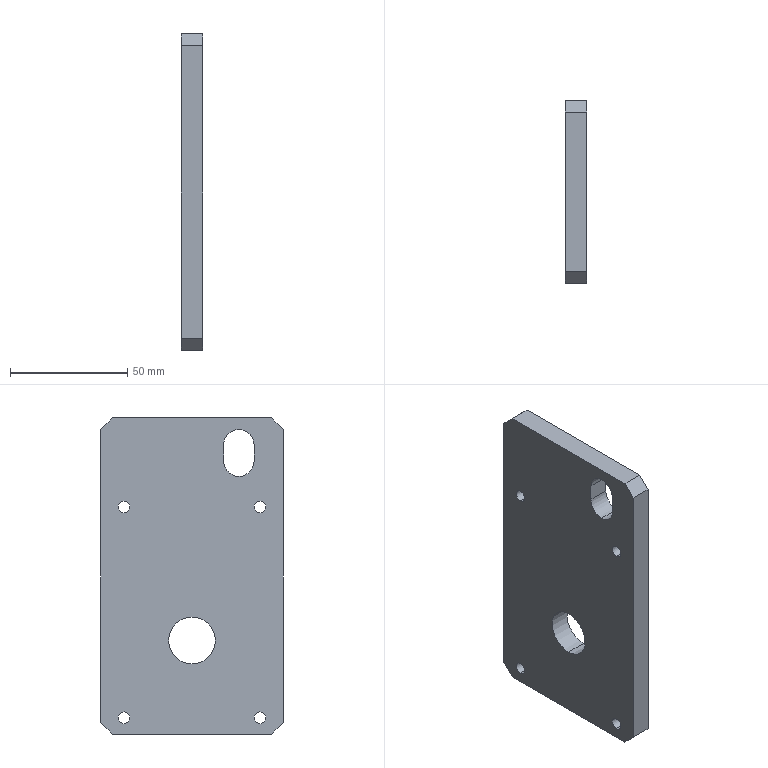Part | STEP file | 0228_213_Arm | 1 solid | 25 faces | box 9 x 78 x 135 mm | volume 88772 mm3 | cylinder 13 | plane 12 | commonest cylinder face diameters 5 x8 13 x3 20 x2